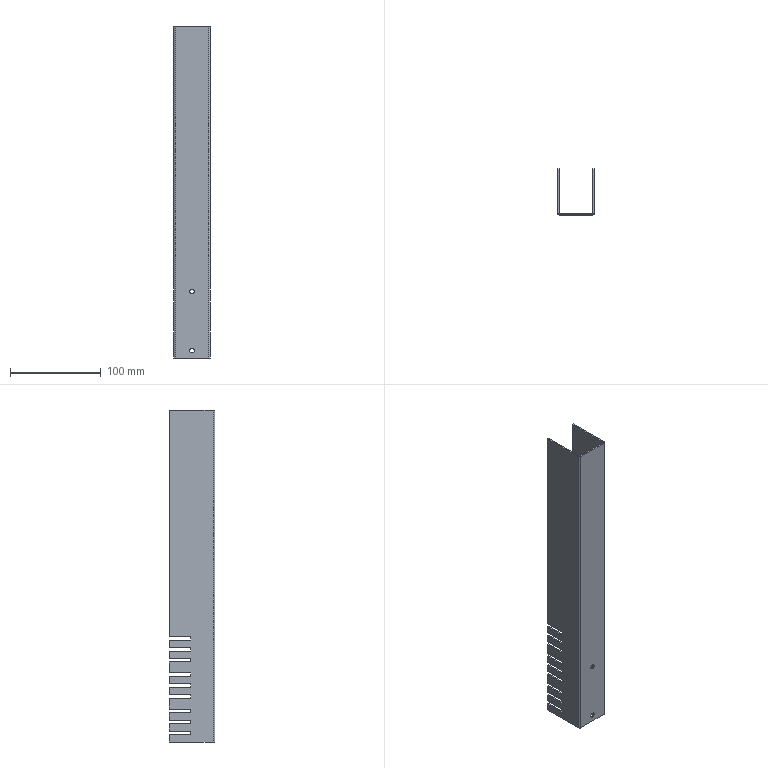Part | SolidWorks | features Cut 1, FlatPattern 1, ICE 1, LPattern 1, SMBaseFlange 1, SheetMetal 1 | 1 solid | 98 faces | box 40 x 50 x 365 mm | volume 71975 mm3 | plane 90 | cylinder 8 | commonest cylinder face diameters 5 x4 0.4 x2 3.4 x2